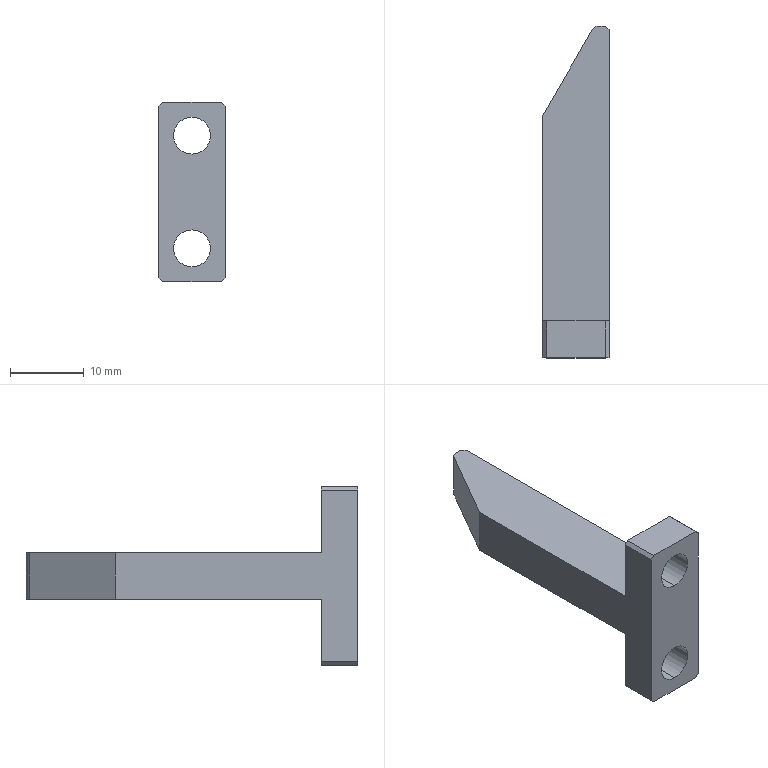Part | SolidWorks | features ICE 3, Chamfer 2, Extrusion 1, Fillet 1 | 1 solid | 21 faces | box 9 x 45 x 24.3 mm | volume 2894 mm3 | plane 16 | cylinder 5 | commonest cylinder face diameters 5 x4 2 x1
STEP:
#1=CARTESIAN_POINT('',(0.,-25.,8.3));
#2=VERTEX_POINT('',#1);
#3=CARTESIAN_POINT('',(0.,-25.,13.3));
#4=VERTEX_POINT('',#3);
#5=CARTESIAN_POINT('',(0.,-25.,10.8));
#6=DIRECTION('',(0.,1.,0.));
#7=DIRECTION('',(0.,0.,1.));
#8=AXIS2_PLACEMENT_3D('',#5,#6,#7);
#9=CIRCLE('',#8,2.5);
#10=EDGE_CURVE('',#2,#4,#9,.T.);
#11=ORIENTED_EDGE('',*,*,#10,.F.);
#12=CARTESIAN_POINT('',(0.,-20.,8.3));
#13=VERTEX_POINT('',#12);
#14=CARTESIAN_POINT('',(0.,-25.,8.3));
#15=DIRECTION('',(0.,1.,0.));
#16=VECTOR('',#15,1000.);
#17=LINE('',#14,#16);
#18=EDGE_CURVE('',#2,#13,#17,.T.);
#19=ORIENTED_EDGE('',*,*,#18,.T.);
#20=CARTESIAN_POINT('',(0.,-20.,13.3));
#21=VERTEX_POINT('',#20);
#22=CARTESIAN_POINT('',(0.,-20.,10.8));
#23=DIRECTION('',(0.,1.,0.));
#24=DIRECTION('',(0.,0.,1.));
#25=AXIS2_PLACEMENT_3D('',#22,#23,#24);
#26=CIRCLE('',#25,2.5);
#27=EDGE_CURVE('',#13,#21,#26,.T.);
#28=ORIENTED_EDGE('',*,*,#27,.T.);
#29=CARTESIAN_POINT('',(0.,-25.,13.3));
#30=DIRECTION('',(0.,1.,0.));
#31=VECTOR('',#30,1000.);
#32=LINE('',#29,#31);
#33=EDGE_CURVE('',#4,#21,#32,.T.);
#34=ORIENTED_EDGE('',*,*,#33,.F.);
#35=EDGE_LOOP('',(#11,#19,#28,#34));
#36=FACE_OUTER_BOUND('',#35,.T.);
#37=CARTESIAN_POINT('',(0.,-25.,10.8));
#38=DIRECTION('',(0.,1.,0.));
#39=DIRECTION('',(0.,0.,1.));
#40=AXIS2_PLACEMENT_3D('',#37,#38,#39);
#41=CYLINDRICAL_SURFACE('',#40,2.5);
#42=ADVANCED_FACE('',(#36),#41,.F.);
#43=CARTESIAN_POINT('',(0.,-25.,-7.));
#44=VERTEX_POINT('',#43);
#45=CARTESIAN_POINT('',(0.,-25.,-2.));
#46=VERTEX_POINT('',#45);
#47=CARTESIAN_POINT('',(0.,-25.,-4.5));
#48=DIRECTION('',(0.,1.,0.));
#49=DIRECTION('',(0.,0.,1.));
#50=AXIS2_PLACEMENT_3D('',#47,#48,#49);
#51=CIRCLE('',#50,2.5);
#52=EDGE_CURVE('',#44,#46,#51,.T.);
#53=ORIENTED_EDGE('',*,*,#52,.F.);
#54=CARTESIAN_POINT('',(0.,-20.,-7.));
#55=VERTEX_POINT('',#54);
#56=CARTESIAN_POINT('',(0.,-25.,-7.));
#57=DIRECTION('',(0.,1.,0.));
#58=VECTOR('',#57,1000.);
#59=LINE('',#56,#58);
#60=EDGE_CURVE('',#44,#55,#59,.T.);
#61=ORIENTED_EDGE('',*,*,#60,.T.);
#62=CARTESIAN_POINT('',(0.,-20.,-2.));
#63=VERTEX_POINT('',#62);
#64=CARTESIAN_POINT('',(0.,-20.,-4.5));
#65=DIRECTION('',(0.,1.,0.));
#66=DIRECTION('',(0.,0.,1.));
#67=AXIS2_PLACEMENT_3D('',#64,#65,#66);
#68=CIRCLE('',#67,2.5);
#69=EDGE_CURVE('',#55,#63,#68,.T.);
#70=ORIENTED_EDGE('',*,*,#69,.T.);
#71=CARTESIAN_POINT('',(0.,-25.,-2.));
#72=DIRECTION('',(0.,1.,0.));
#73=VECTOR('',#72,1000.);
#74=LINE('',#71,#73);
#75=EDGE_CURVE('',#46,#63,#74,.T.);
#76=ORIENTED_EDGE('',*,*,#75,.F.);
#77=EDGE_LOOP('',(#53,#61,#70,#76));
#78=FACE_OUTER_BOUND('',#77,.T.);
#79=CARTESIAN_POINT('',(0.,-25.,-4.5));
#80=DIRECTION('',(0.,1.,0.));
#81=DIRECTION('',(0.,0.,1.));
#82=AXIS2_PLACEMENT_3D('',#79,#80,#81);
#83=CYLINDRICAL_SURFACE('',#82,2.5);
#84=ADVANCED_FACE('',(#78),#83,.F.);
#85=CARTESIAN_POINT('',(4.5,-20.,0.));
#86=VERTEX_POINT('',#85);
#87=CARTESIAN_POINT('',(4.5,19.5,0.));
#88=VERTEX_POINT('',#87);
#89=CARTESIAN_POINT('',(4.5,20.,0.));
#90=DIRECTION('',(0.,1.,0.));
#91=VECTOR('',#90,1000.);
#92=LINE('',#89,#91);
#93=EDGE_CURVE('',#86,#88,#92,.T.);
#94=ORIENTED_EDGE('',*,*,#93,.T.);
#95=CARTESIAN_POINT('',(4.5,19.5,6.3));
#96=VERTEX_POINT('',#95);
#97=CARTESIAN_POINT('',(4.5,19.5,6.3));
#98=DIRECTION('',(0.,0.,1.));
#99=VECTOR('',#98,1000.);
#100=LINE('',#97,#99);
#101=EDGE_CURVE('',#88,#96,#100,.T.);
#102=ORIENTED_EDGE('',*,*,#101,.T.);
#103=CARTESIAN_POINT('',(4.5,-20.,6.3));
#104=VERTEX_POINT('',#103);
#105=CARTESIAN_POINT('',(4.5,20.,6.3));
#106=DIRECTION('',(0.,1.,0.));
#107=VECTOR('',#106,1000.);
#108=LINE('',#105,#107);
#109=EDGE_CURVE('',#104,#96,#108,.T.);
#110=ORIENTED_EDGE('',*,*,#109,.F.);
#111=CARTESIAN_POINT('',(4.5,-20.,14.8));
#112=VERTEX_POINT('',#111);
#113=CARTESIAN_POINT('',(4.5,-20.,15.3));
#114=DIRECTION('',(0.,0.,1.));
#115=VECTOR('',#114,1000.);
#116=LINE('',#113,#115);
#117=EDGE_CURVE('',#104,#112,#116,.T.);
#118=ORIENTED_EDGE('',*,*,#117,.T.);
#119=CARTESIAN_POINT('',(4.5,-25.,14.8));
#120=VERTEX_POINT('',#119);
#121=CARTESIAN_POINT('',(4.5,20.,14.8));
#122=DIRECTION('',(0.,-1.,0.));
#123=VECTOR('',#122,1000.);
#124=LINE('',#121,#123);
#125=EDGE_CURVE('',#112,#120,#124,.T.);
#126=ORIENTED_EDGE('',*,*,#125,.T.);
#127=CARTESIAN_POINT('',(4.5,-25.,-8.5));
#128=VERTEX_POINT('',#127);
#129=CARTESIAN_POINT('',(4.5,-25.,15.3));
#130=DIRECTION('',(0.,0.,1.));
#131=VECTOR('',#130,1000.);
#132=LINE('',#129,#131);
#133=EDGE_CURVE('',#128,#120,#132,.T.);
#134=ORIENTED_EDGE('',*,*,#133,.F.);
#135=CARTESIAN_POINT('',(4.5,-20.,-8.5));
#136=VERTEX_POINT('',#135);
#137=CARTESIAN_POINT('',(4.5,20.,-8.5));
#138=DIRECTION('',(0.,1.,0.));
#139=VECTOR('',#138,1000.);
#140=LINE('',#137,#139);
#141=EDGE_CURVE('',#128,#136,#140,.T.);
#142=ORIENTED_EDGE('',*,*,#141,.T.);
#143=CARTESIAN_POINT('',(4.5,-20.,15.3));
#144=DIRECTION('',(0.,0.,1.));
#145=VECTOR('',#144,1000.);
#146=LINE('',#143,#145);
#147=EDGE_CURVE('',#136,#86,#146,.T.);
#148=ORIENTED_EDGE('',*,*,#147,.T.);
#149=EDGE_LOOP('',(#94,#102,#110,#118,#126,#134,#142,#148));
#150=FACE_OUTER_BOUND('',#149,.T.);
#151=CARTESIAN_POINT('',(4.5,20.,6.3));
#152=DIRECTION('',(-1.,0.,0.));
#153=DIRECTION('',(0.,-1.,0.));
#154=AXIS2_PLACEMENT_3D('',#151,#152,#153);
#155=PLANE('',#154);
#156=ADVANCED_FACE('',(#150),#155,.F.);
#157=CARTESIAN_POINT('',(4.,20.,6.3));
#158=VERTEX_POINT('',#157);
#159=CARTESIAN_POINT('',(3.077,20.,6.3));
#160=VERTEX_POINT('',#159);
#161=CARTESIAN_POINT('',(-4.5,20.,6.3));
#162=DIRECTION('',(-1.,0.,0.));
#163=VECTOR('',#162,1000.);
#164=LINE('',#161,#163);
#165=EDGE_CURVE('',#158,#160,#164,.T.);
#166=ORIENTED_EDGE('',*,*,#165,.F.);
#167=CARTESIAN_POINT('',(4.,20.,0.));
#168=VERTEX_POINT('',#167);
#169=CARTESIAN_POINT('',(4.,20.,6.3));
#170=DIRECTION('',(0.,0.,-1.));
#171=VECTOR('',#170,1000.);
#172=LINE('',#169,#171);
#173=EDGE_CURVE('',#158,#168,#172,.T.);
#174=ORIENTED_EDGE('',*,*,#173,.T.);
#175=CARTESIAN_POINT('',(3.077,20.,0.));
#176=VERTEX_POINT('',#175);
#177=CARTESIAN_POINT('',(-4.5,20.,0.));
#178=DIRECTION('',(-1.,0.,0.));
#179=VECTOR('',#178,1000.);
#180=LINE('',#177,#179);
#181=EDGE_CURVE('',#168,#176,#180,.T.);
#182=ORIENTED_EDGE('',*,*,#181,.T.);
#183=CARTESIAN_POINT('',(3.077,20.,6.3));
#184=DIRECTION('',(0.,0.,1.));
#185=VECTOR('',#184,1000.);
#186=LINE('',#183,#185);
#187=EDGE_CURVE('',#176,#160,#186,.T.);
#188=ORIENTED_EDGE('',*,*,#187,.T.);
#189=EDGE_LOOP('',(#166,#174,#182,#188));
#190=FACE_OUTER_BOUND('',#189,.T.);
#191=CARTESIAN_POINT('',(-4.5,20.,6.3));
#192=DIRECTION('',(0.,-1.,0.));
#193=DIRECTION('',(0.,0.,-1.));
#194=AXIS2_PLACEMENT_3D('',#191,#192,#193);
#195=PLANE('',#194);
#196=ADVANCED_FACE('',(#190),#195,.F.);
#197=CARTESIAN_POINT('',(-4.5,-20.,0.));
#198=VERTEX_POINT('',#197);
#199=CARTESIAN_POINT('',(-4.5,-20.,-8.5));
#200=VERTEX_POINT('',#199);
#201=CARTESIAN_POINT('',(-4.5,-20.,15.3));
#202=DIRECTION('',(0.,0.,-1.));
#203=VECTOR('',#202,1000.);
#204=LINE('',#201,#203);
#205=EDGE_CURVE('',#198,#200,#204,.T.);
#206=ORIENTED_EDGE('',*,*,#205,.T.);
#207=CARTESIAN_POINT('',(-4.5,-25.,-8.5));
#208=VERTEX_POINT('',#207);
#209=CARTESIAN_POINT('',(-4.5,20.,-8.5));
#210=DIRECTION('',(0.,-1.,0.));
#211=VECTOR('',#210,1000.);
#212=LINE('',#209,#211);
#213=EDGE_CURVE('',#200,#208,#212,.T.);
#214=ORIENTED_EDGE('',*,*,#213,.T.);
#215=CARTESIAN_POINT('',(-4.5,-25.,14.8));
#216=VERTEX_POINT('',#215);
#217=CARTESIAN_POINT('',(-4.5,-25.,15.3));
#218=DIRECTION('',(0.,0.,-1.));
#219=VECTOR('',#218,1000.);
#220=LINE('',#217,#219);
#221=EDGE_CURVE('',#216,#208,#220,.T.);
#222=ORIENTED_EDGE('',*,*,#221,.F.);
#223=CARTESIAN_POINT('',(-4.5,-20.,14.8));
#224=VERTEX_POINT('',#223);
#225=CARTESIAN_POINT('',(-4.5,20.,14.8));
#226=DIRECTION('',(0.,1.,0.));
#227=VECTOR('',#226,1000.);
#228=LINE('',#225,#227);
#229=EDGE_CURVE('',#216,#224,#228,.T.);
#230=ORIENTED_EDGE('',*,*,#229,.T.);
#231=CARTESIAN_POINT('',(-4.5,-20.,6.3));
#232=VERTEX_POINT('',#231);
#233=CARTESIAN_POINT('',(-4.5,-20.,15.3));
#234=DIRECTION('',(0.,0.,-1.));
#235=VECTOR('',#234,1000.);
#236=LINE('',#233,#235);
#237=EDGE_CURVE('',#224,#232,#236,.T.);
#238=ORIENTED_EDGE('',*,*,#237,.T.);
#239=CARTESIAN_POINT('',(-4.5,7.876,6.3));
#240=VERTEX_POINT('',#239);
#241=CARTESIAN_POINT('',(-4.5,20.,6.3));
#242=DIRECTION('',(0.,-1.,0.));
#243=VECTOR('',#242,1000.);
#244=LINE('',#241,#243);
#245=EDGE_CURVE('',#240,#232,#244,.T.);
#246=ORIENTED_EDGE('',*,*,#245,.F.);
#247=CARTESIAN_POINT('',(-4.5,7.876,0.));
#248=VERTEX_POINT('',#247);
#249=CARTESIAN_POINT('',(-4.5,7.876,15.3));
#250=DIRECTION('',(0.,0.,-1.));
#251=VECTOR('',#250,1000.);
#252=LINE('',#249,#251);
#253=EDGE_CURVE('',#240,#248,#252,.T.);
#254=ORIENTED_EDGE('',*,*,#253,.T.);
#255=CARTESIAN_POINT('',(-4.5,20.,0.));
#256=DIRECTION('',(0.,-1.,0.));
#257=VECTOR('',#256,1000.);
#258=LINE('',#255,#257);
#259=EDGE_CURVE('',#248,#198,#258,.T.);
#260=ORIENTED_EDGE('',*,*,#259,.T.);
#261=EDGE_LOOP('',(#206,#214,#222,#230,#238,#246,#254,#260));
#262=FACE_OUTER_BOUND('',#261,.T.);
#263=CARTESIAN_POINT('',(-4.5,20.,6.3));
#264=DIRECTION('',(1.,0.,0.));
#265=DIRECTION('',(0.,1.,0.));
#266=AXIS2_PLACEMENT_3D('',#263,#264,#265);
#267=PLANE('',#266);
#268=ADVANCED_FACE('',(#262),#267,.F.);
#269=ORIENTED_EDGE('',*,*,#109,.T.);
#270=CARTESIAN_POINT('',(12.,12.,6.3));
#271=DIRECTION('',(-0.7071,0.7071,0.));
#272=VECTOR('',#271,1000.);
#273=LINE('',#270,#272);
#274=EDGE_CURVE('',#96,#158,#273,.T.);
#275=ORIENTED_EDGE('',*,*,#274,.T.);
#276=ORIENTED_EDGE('',*,*,#165,.T.);
#277=CARTESIAN_POINT('',(2.211,19.5,6.3));
#278=VERTEX_POINT('',#277);
#279=CARTESIAN_POINT('',(3.077,19.,6.3));
#280=DIRECTION('',(0.,0.,1.));
#281=DIRECTION('',(1.,0.,0.));
#282=AXIS2_PLACEMENT_3D('',#279,#280,#281);
#283=CIRCLE('',#282,1.);
#284=EDGE_CURVE('',#160,#278,#283,.T.);
#285=ORIENTED_EDGE('',*,*,#284,.T.);
#286=CARTESIAN_POINT('',(-6.785,3.917,6.3));
#287=DIRECTION('',(0.5,0.866,0.));
#288=VECTOR('',#287,1000.);
#289=LINE('',#286,#288);
#290=EDGE_CURVE('',#240,#278,#289,.T.);
#291=ORIENTED_EDGE('',*,*,#290,.F.);
#292=ORIENTED_EDGE('',*,*,#245,.T.);
#293=CARTESIAN_POINT('',(-4.5,-20.,6.3));
#294=DIRECTION('',(1.,0.,0.));
#295=VECTOR('',#294,1000.);
#296=LINE('',#293,#295);
#297=EDGE_CURVE('',#232,#104,#296,.T.);
#298=ORIENTED_EDGE('',*,*,#297,.T.);
#299=EDGE_LOOP('',(#269,#275,#276,#285,#291,#292,#298));
#300=FACE_OUTER_BOUND('',#299,.T.);
#301=CARTESIAN_POINT('',(0.,0.,6.3));
#302=DIRECTION('',(0.,0.,1.));
#303=DIRECTION('',(1.,0.,0.));
#304=AXIS2_PLACEMENT_3D('',#301,#302,#303);
#305=PLANE('',#304);
#306=ADVANCED_FACE('',(#300),#305,.T.);
#307=ORIENTED_EDGE('',*,*,#181,.F.);
#308=CARTESIAN_POINT('',(4.,20.,0.));
#309=DIRECTION('',(0.7071,-0.7071,0.));
#310=VECTOR('',#309,1000.);
#311=LINE('',#308,#310);
#312=EDGE_CURVE('',#168,#88,#311,.T.);
#313=ORIENTED_EDGE('',*,*,#312,.T.);
#314=ORIENTED_EDGE('',*,*,#93,.F.);
#315=CARTESIAN_POINT('',(-4.5,-20.,0.));
#316=DIRECTION('',(1.,0.,0.));
#317=VECTOR('',#316,1000.);
#318=LINE('',#315,#317);
#319=EDGE_CURVE('',#198,#86,#318,.T.);
#320=ORIENTED_EDGE('',*,*,#319,.F.);
#321=ORIENTED_EDGE('',*,*,#259,.F.);
#322=CARTESIAN_POINT('',(2.211,19.5,0.));
#323=VERTEX_POINT('',#322);
#324=CARTESIAN_POINT('',(-4.5,7.876,0.));
#325=DIRECTION('',(-0.5,-0.866,0.));
#326=VECTOR('',#325,1000.);
#327=LINE('',#324,#326);
#328=EDGE_CURVE('',#323,#248,#327,.T.);
#329=ORIENTED_EDGE('',*,*,#328,.F.);
#330=CARTESIAN_POINT('',(3.077,19.,0.));
#331=DIRECTION('',(0.,0.,-1.));
#332=DIRECTION('',(1.,0.,0.));
#333=AXIS2_PLACEMENT_3D('',#330,#331,#332);
#334=CIRCLE('',#333,1.);
#335=EDGE_CURVE('',#323,#176,#334,.T.);
#336=ORIENTED_EDGE('',*,*,#335,.T.);
#337=EDGE_LOOP('',(#307,#313,#314,#320,#321,#329,#336));
#338=FACE_OUTER_BOUND('',#337,.T.);
#339=CARTESIAN_POINT('',(0.,0.,0.));
#340=DIRECTION('',(0.,0.,1.));
#341=DIRECTION('',(1.,0.,0.));
#342=AXIS2_PLACEMENT_3D('',#339,#340,#341);
#343=PLANE('',#342);
#344=ADVANCED_FACE('',(#338),#343,.F.);
#345=CARTESIAN_POINT('',(0.,-20.,-4.5));
#346=DIRECTION('',(0.,1.,0.));
#347=DIRECTION('',(0.,0.,1.));
#348=AXIS2_PLACEMENT_3D('',#345,#346,#347);
#349=CIRCLE('',#348,2.5);
#350=EDGE_CURVE('',#63,#55,#349,.T.);
#351=ORIENTED_EDGE('',*,*,#350,.F.);
#352=ORIENTED_EDGE('',*,*,#69,.F.);
#353=EDGE_LOOP('',(#351,#352));
#354=FACE_BOUND('',#353,.T.);
#355=ORIENTED_EDGE('',*,*,#147,.F.);
#356=CARTESIAN_POINT('',(4.,-20.,-9.));
#357=VERTEX_POINT('',#356);
#358=CARTESIAN_POINT('',(4.5,-20.,-8.5));
#359=DIRECTION('',(-0.7071,0.,-0.7071));
#360=VECTOR('',#359,1000.);
#361=LINE('',#358,#360);
#362=EDGE_CURVE('',#136,#357,#361,.T.);
#363=ORIENTED_EDGE('',*,*,#362,.T.);
#364=CARTESIAN_POINT('',(-4.,-20.,-9.));
#365=VERTEX_POINT('',#364);
#366=CARTESIAN_POINT('',(-4.5,-20.,-9.));
#367=DIRECTION('',(1.,0.,0.));
#368=VECTOR('',#367,1000.);
#369=LINE('',#366,#368);
#370=EDGE_CURVE('',#365,#357,#369,.T.);
#371=ORIENTED_EDGE('',*,*,#370,.F.);
#372=CARTESIAN_POINT('',(-4.,-20.,-9.));
#373=DIRECTION('',(-0.7071,0.,0.7071));
#374=VECTOR('',#373,1000.);
#375=LINE('',#372,#374);
#376=EDGE_CURVE('',#365,#200,#375,.T.);
#377=ORIENTED_EDGE('',*,*,#376,.T.);
#378=ORIENTED_EDGE('',*,*,#205,.F.);
#379=ORIENTED_EDGE('',*,*,#319,.T.);
#380=EDGE_LOOP('',(#355,#363,#371,#377,#378,#379));
#381=FACE_OUTER_BOUND('',#380,.T.);
#382=CARTESIAN_POINT('',(0.,-20.,0.));
#383=DIRECTION('',(0.,-1.,0.));
#384=DIRECTION('',(0.,0.,-1.));
#385=AXIS2_PLACEMENT_3D('',#382,#383,#384);
#386=PLANE('',#385);
#387=ADVANCED_FACE('',(#354,#381),#386,.F.);
#388=ORIENTED_EDGE('',*,*,#370,.T.);
#389=CARTESIAN_POINT('',(4.,-25.,-9.));
#390=VERTEX_POINT('',#389);
#391=CARTESIAN_POINT('',(4.,-25.,-9.));
#392=DIRECTION('',(0.,-1.,0.));
#393=VECTOR('',#392,1000.);
#394=LINE('',#391,#393);
#395=EDGE_CURVE('',#357,#390,#394,.T.);
#396=ORIENTED_EDGE('',*,*,#395,.T.);
#397=CARTESIAN_POINT('',(-4.,-25.,-9.));
#398=VERTEX_POINT('',#397);
#399=CARTESIAN_POINT('',(-4.5,-25.,-9.));
#400=DIRECTION('',(1.,0.,0.));
#401=VECTOR('',#400,1000.);
#402=LINE('',#399,#401);
#403=EDGE_CURVE('',#398,#390,#402,.T.);
#404=ORIENTED_EDGE('',*,*,#403,.F.);
#405=CARTESIAN_POINT('',(-4.,-25.,-9.));
#406=DIRECTION('',(0.,1.,0.));
#407=VECTOR('',#406,1000.);
#408=LINE('',#405,#407);
#409=EDGE_CURVE('',#398,#365,#408,.T.);
#410=ORIENTED_EDGE('',*,*,#409,.T.);
#411=EDGE_LOOP('',(#388,#396,#404,#410));
#412=FACE_OUTER_BOUND('',#411,.T.);
#413=CARTESIAN_POINT('',(-4.5,-25.,-9.));
#414=DIRECTION('',(0.,0.,1.));
#415=DIRECTION('',(1.,0.,0.));
#416=AXIS2_PLACEMENT_3D('',#413,#414,#415);
#417=PLANE('',#416);
#418=ADVANCED_FACE('',(#412),#417,.F.);
#419=CARTESIAN_POINT('',(4.,-25.,15.3));
#420=VERTEX_POINT('',#419);
#421=CARTESIAN_POINT('',(-4.,-25.,15.3));
#422=VERTEX_POINT('',#421);
#423=CARTESIAN_POINT('',(-4.5,-25.,15.3));
#424=DIRECTION('',(-1.,0.,0.));
#425=VECTOR('',#424,1000.);
#426=LINE('',#423,#425);
#427=EDGE_CURVE('',#420,#422,#426,.T.);
#428=ORIENTED_EDGE('',*,*,#427,.F.);
#429=CARTESIAN_POINT('',(4.,-20.,15.3));
#430=VERTEX_POINT('',#429);
#431=CARTESIAN_POINT('',(4.,-25.,15.3));
#432=DIRECTION('',(0.,1.,0.));
#433=VECTOR('',#432,1000.);
#434=LINE('',#431,#433);
#435=EDGE_CURVE('',#420,#430,#434,.T.);
#436=ORIENTED_EDGE('',*,*,#435,.T.);
#437=CARTESIAN_POINT('',(-4.,-20.,15.3));
#438=VERTEX_POINT('',#437);
#439=CARTESIAN_POINT('',(-4.5,-20.,15.3));
#440=DIRECTION('',(-1.,0.,0.));
#441=VECTOR('',#440,1000.);
#442=LINE('',#439,#441);
#443=EDGE_CURVE('',#430,#438,#442,.T.);
#444=ORIENTED_EDGE('',*,*,#443,.T.);
#445=CARTESIAN_POINT('',(-4.,-25.,15.3));
#446=DIRECTION('',(0.,-1.,0.));
#447=VECTOR('',#446,1000.);
#448=LINE('',#445,#447);
#449=EDGE_CURVE('',#438,#422,#448,.T.);
#450=ORIENTED_EDGE('',*,*,#449,.T.);
#451=EDGE_LOOP('',(#428,#436,#444,#450));
#452=FACE_OUTER_BOUND('',#451,.T.);
#453=CARTESIAN_POINT('',(-4.5,-25.,15.3));
#454=DIRECTION('',(0.,0.,-1.));
#455=DIRECTION('',(-1.,0.,0.));
#456=AXIS2_PLACEMENT_3D('',#453,#454,#455);
#457=PLANE('',#456);
#458=ADVANCED_FACE('',(#452),#457,.F.);
#459=CARTESIAN_POINT('',(0.,-25.,10.8));
#460=DIRECTION('',(0.,1.,0.));
#461=DIRECTION('',(0.,0.,1.));
#462=AXIS2_PLACEMENT_3D('',#459,#460,#461);
#463=CIRCLE('',#462,2.5);
#464=EDGE_CURVE('',#4,#2,#463,.T.);
#465=ORIENTED_EDGE('',*,*,#464,.T.);
#466=ORIENTED_EDGE('',*,*,#10,.T.);
#467=EDGE_LOOP('',(#465,#466));
#468=FACE_BOUND('',#467,.T.);
#469=CARTESIAN_POINT('',(0.,-25.,-4.5));
#470=DIRECTION('',(0.,1.,0.));
#471=DIRECTION('',(0.,0.,1.));
#472=AXIS2_PLACEMENT_3D('',#469,#470,#471);
#473=CIRCLE('',#472,2.5);
#474=EDGE_CURVE('',#46,#44,#473,.T.);
#475=ORIENTED_EDGE('',*,*,#474,.T.);
#476=ORIENTED_EDGE('',*,*,#52,.T.);
#477=EDGE_LOOP('',(#475,#476));
#478=FACE_BOUND('',#477,.T.);
#479=ORIENTED_EDGE('',*,*,#403,.T.);
#480=CARTESIAN_POINT('',(6.5,-25.,-6.5));
#481=DIRECTION('',(0.7071,0.,0.7071));
#482=VECTOR('',#481,1000.);
#483=LINE('',#480,#482);
#484=EDGE_CURVE('',#390,#128,#483,.T.);
#485=ORIENTED_EDGE('',*,*,#484,.T.);
#486=ORIENTED_EDGE('',*,*,#133,.T.);
#487=CARTESIAN_POINT('',(9.65,-25.,9.65));
#488=DIRECTION('',(-0.7071,0.,0.7071));
#489=VECTOR('',#488,1000.);
#490=LINE('',#487,#489);
#491=EDGE_CURVE('',#120,#420,#490,.T.);
#492=ORIENTED_EDGE('',*,*,#491,.T.);
#493=ORIENTED_EDGE('',*,*,#427,.T.);
#494=CARTESIAN_POINT('',(-9.65,-25.,9.65));
#495=DIRECTION('',(-0.7071,0.,-0.7071));
#496=VECTOR('',#495,1000.);
#497=LINE('',#494,#496);
#498=EDGE_CURVE('',#422,#216,#497,.T.);
#499=ORIENTED_EDGE('',*,*,#498,.T.);
#500=ORIENTED_EDGE('',*,*,#221,.T.);
#501=CARTESIAN_POINT('',(-6.5,-25.,-6.5));
#502=DIRECTION('',(0.7071,0.,-0.7071));
#503=VECTOR('',#502,1000.);
#504=LINE('',#501,#503);
#505=EDGE_CURVE('',#208,#398,#504,.T.);
#506=ORIENTED_EDGE('',*,*,#505,.T.);
#507=EDGE_LOOP('',(#479,#485,#486,#492,#493,#499,#500,#506));
#508=FACE_OUTER_BOUND('',#507,.T.);
#509=CARTESIAN_POINT('',(0.,-25.,0.));
#510=DIRECTION('',(0.,-1.,0.));
#511=DIRECTION('',(0.,0.,-1.));
#512=AXIS2_PLACEMENT_3D('',#509,#510,#511);
#513=PLANE('',#512);
#514=ADVANCED_FACE('',(#468,#478,#508),#513,.T.);
#515=CARTESIAN_POINT('',(0.,-20.,10.8));
#516=DIRECTION('',(0.,1.,0.));
#517=DIRECTION('',(0.,0.,1.));
#518=AXIS2_PLACEMENT_3D('',#515,#516,#517);
#519=CIRCLE('',#518,2.5);
#520=EDGE_CURVE('',#21,#13,#519,.T.);
#521=ORIENTED_EDGE('',*,*,#520,.F.);
#522=ORIENTED_EDGE('',*,*,#27,.F.);
#523=EDGE_LOOP('',(#521,#522));
#524=FACE_BOUND('',#523,.T.);
#525=ORIENTED_EDGE('',*,*,#443,.F.);
#526=CARTESIAN_POINT('',(4.,-20.,15.3));
#527=DIRECTION('',(0.7071,0.,-0.7071));
#528=VECTOR('',#527,1000.);
#529=LINE('',#526,#528);
#530=EDGE_CURVE('',#430,#112,#529,.T.);
#531=ORIENTED_EDGE('',*,*,#530,.T.);
#532=ORIENTED_EDGE('',*,*,#117,.F.);
#533=ORIENTED_EDGE('',*,*,#297,.F.);
#534=ORIENTED_EDGE('',*,*,#237,.F.);
#535=CARTESIAN_POINT('',(-4.5,-20.,14.8));
#536=DIRECTION('',(0.7071,0.,0.7071));
#537=VECTOR('',#536,1000.);
#538=LINE('',#535,#537);
#539=EDGE_CURVE('',#224,#438,#538,.T.);
#540=ORIENTED_EDGE('',*,*,#539,.T.);
#541=EDGE_LOOP('',(#525,#531,#532,#533,#534,#540));
#542=FACE_OUTER_BOUND('',#541,.T.);
#543=CARTESIAN_POINT('',(0.,-20.,0.));
#544=DIRECTION('',(0.,-1.,0.));
#545=DIRECTION('',(0.,0.,-1.));
#546=AXIS2_PLACEMENT_3D('',#543,#544,#545);
#547=PLANE('',#546);
#548=ADVANCED_FACE('',(#524,#542),#547,.F.);
#549=ORIENTED_EDGE('',*,*,#290,.T.);
#550=CARTESIAN_POINT('',(2.211,19.5,15.3));
#551=DIRECTION('',(0.,0.,-1.));
#552=VECTOR('',#551,1000.);
#553=LINE('',#550,#552);
#554=EDGE_CURVE('',#278,#323,#553,.T.);
#555=ORIENTED_EDGE('',*,*,#554,.T.);
#556=ORIENTED_EDGE('',*,*,#328,.T.);
#557=ORIENTED_EDGE('',*,*,#253,.F.);
#558=EDGE_LOOP('',(#549,#555,#556,#557));
#559=FACE_OUTER_BOUND('',#558,.T.);
#560=CARTESIAN_POINT('',(-4.5,7.876,15.3));
#561=DIRECTION('',(0.866,-0.5,0.));
#562=DIRECTION('',(0.5,0.866,0.));
#563=AXIS2_PLACEMENT_3D('',#560,#561,#562);
#564=PLANE('',#563);
#565=ADVANCED_FACE('',(#559),#564,.F.);
#566=ORIENTED_EDGE('',*,*,#60,.F.);
#567=ORIENTED_EDGE('',*,*,#474,.F.);
#568=ORIENTED_EDGE('',*,*,#75,.T.);
#569=ORIENTED_EDGE('',*,*,#350,.T.);
#570=EDGE_LOOP('',(#566,#567,#568,#569));
#571=FACE_OUTER_BOUND('',#570,.T.);
#572=CARTESIAN_POINT('',(0.,-25.,-4.5));
#573=DIRECTION('',(0.,1.,0.));
#574=DIRECTION('',(0.,0.,1.));
#575=AXIS2_PLACEMENT_3D('',#572,#573,#574);
#576=CYLINDRICAL_SURFACE('',#575,2.5);
#577=ADVANCED_FACE('',(#571),#576,.F.);
#578=ORIENTED_EDGE('',*,*,#18,.F.);
#579=ORIENTED_EDGE('',*,*,#464,.F.);
#580=ORIENTED_EDGE('',*,*,#33,.T.);
#581=ORIENTED_EDGE('',*,*,#520,.T.);
#582=EDGE_LOOP('',(#578,#579,#580,#581));
#583=FACE_OUTER_BOUND('',#582,.T.);
#584=CARTESIAN_POINT('',(0.,-25.,10.8));
#585=DIRECTION('',(0.,1.,0.));
#586=DIRECTION('',(0.,0.,1.));
#587=AXIS2_PLACEMENT_3D('',#584,#585,#586);
#588=CYLINDRICAL_SURFACE('',#587,2.5);
#589=ADVANCED_FACE('',(#583),#588,.F.);
#590=ORIENTED_EDGE('',*,*,#284,.F.);
#591=ORIENTED_EDGE('',*,*,#187,.F.);
#592=ORIENTED_EDGE('',*,*,#335,.F.);
#593=ORIENTED_EDGE('',*,*,#554,.F.);
#594=EDGE_LOOP('',(#590,#591,#592,#593));
#595=FACE_OUTER_BOUND('',#594,.T.);
#596=CARTESIAN_POINT('',(3.077,19.,15.3));
#597=DIRECTION('',(0.,0.,-1.));
#598=DIRECTION('',(-1.,0.,0.));
#599=AXIS2_PLACEMENT_3D('',#596,#597,#598);
#600=CYLINDRICAL_SURFACE('',#599,1.);
#601=ADVANCED_FACE('',(#595),#600,.T.);
#602=ORIENTED_EDGE('',*,*,#274,.F.);
#603=ORIENTED_EDGE('',*,*,#101,.F.);
#604=ORIENTED_EDGE('',*,*,#312,.F.);
#605=ORIENTED_EDGE('',*,*,#173,.F.);
#606=EDGE_LOOP('',(#602,#603,#604,#605));
#607=FACE_OUTER_BOUND('',#606,.T.);
#608=CARTESIAN_POINT('',(4.,20.,6.3));
#609=DIRECTION('',(-0.7071,-0.7071,0.));
#610=DIRECTION('',(0.,0.,-1.));
#611=AXIS2_PLACEMENT_3D('',#608,#609,#610);
#612=PLANE('',#611);
#613=ADVANCED_FACE('',(#607),#612,.F.);
#614=ORIENTED_EDGE('',*,*,#484,.F.);
#615=ORIENTED_EDGE('',*,*,#395,.F.);
#616=ORIENTED_EDGE('',*,*,#362,.F.);
#617=ORIENTED_EDGE('',*,*,#141,.F.);
#618=EDGE_LOOP('',(#614,#615,#616,#617));
#619=FACE_OUTER_BOUND('',#618,.T.);
#620=CARTESIAN_POINT('',(4.5,20.,-8.5));
#621=DIRECTION('',(-0.7071,0.,0.7071));
#622=DIRECTION('',(0.,1.,0.));
#623=AXIS2_PLACEMENT_3D('',#620,#621,#622);
#624=PLANE('',#623);
#625=ADVANCED_FACE('',(#619),#624,.F.);
#626=ORIENTED_EDGE('',*,*,#505,.F.);
#627=ORIENTED_EDGE('',*,*,#213,.F.);
#628=ORIENTED_EDGE('',*,*,#376,.F.);
#629=ORIENTED_EDGE('',*,*,#409,.F.);
#630=EDGE_LOOP('',(#626,#627,#628,#629));
#631=FACE_OUTER_BOUND('',#630,.T.);
#632=CARTESIAN_POINT('',(-4.,-25.,-9.));
#633=DIRECTION('',(0.7071,0.,0.7071));
#634=DIRECTION('',(0.,1.,0.));
#635=AXIS2_PLACEMENT_3D('',#632,#633,#634);
#636=PLANE('',#635);
#637=ADVANCED_FACE('',(#631),#636,.F.);
#638=ORIENTED_EDGE('',*,*,#491,.F.);
#639=ORIENTED_EDGE('',*,*,#125,.F.);
#640=ORIENTED_EDGE('',*,*,#530,.F.);
#641=ORIENTED_EDGE('',*,*,#435,.F.);
#642=EDGE_LOOP('',(#638,#639,#640,#641));
#643=FACE_OUTER_BOUND('',#642,.T.);
#644=CARTESIAN_POINT('',(4.,-25.,15.3));
#645=DIRECTION('',(-0.7071,0.,-0.7071));
#646=DIRECTION('',(0.,1.,0.));
#647=AXIS2_PLACEMENT_3D('',#644,#645,#646);
#648=PLANE('',#647);
#649=ADVANCED_FACE('',(#643),#648,.F.);
#650=ORIENTED_EDGE('',*,*,#498,.F.);
#651=ORIENTED_EDGE('',*,*,#449,.F.);
#652=ORIENTED_EDGE('',*,*,#539,.F.);
#653=ORIENTED_EDGE('',*,*,#229,.F.);
#654=EDGE_LOOP('',(#650,#651,#652,#653));
#655=FACE_OUTER_BOUND('',#654,.T.);
#656=CARTESIAN_POINT('',(-4.5,20.,14.8));
#657=DIRECTION('',(0.7071,0.,-0.7071));
#658=DIRECTION('',(0.,1.,0.));
#659=AXIS2_PLACEMENT_3D('',#656,#657,#658);
#660=PLANE('',#659);
#661=ADVANCED_FACE('',(#655),#660,.F.);
#662=CLOSED_SHELL('',(#42,#84,#156,#196,#268,#306,#344,#387,#418,#458,#514,#548,#565,#577,#589,#601,#613,#625,#637,#649,#661));
#663=MANIFOLD_SOLID_BREP('',#662);
#664=CARTESIAN_POINT('',(0.,0.,0.));
#665=DIRECTION('',(0.,0.,1.));
#666=DIRECTION('',(1.,0.,0.));
#667=AXIS2_PLACEMENT_3D('',#664,#665,#666);
#668=(LENGTH_UNIT()NAMED_UNIT(*)SI_UNIT(.MILLI.,.METRE.));
#669=UNCERTAINTY_MEASURE_WITH_UNIT(LENGTH_MEASURE(0.00001),#668,'','');
#670=(NAMED_UNIT(*)PLANE_ANGLE_UNIT()SI_UNIT($,.RADIAN.));
#671=(NAMED_UNIT(*)SI_UNIT($,.STERADIAN.)SOLID_ANGLE_UNIT());
#672=(GEOMETRIC_REPRESENTATION_CONTEXT(3)GLOBAL_UNCERTAINTY_ASSIGNED_CONTEXT((#669))GLOBAL_UNIT_ASSIGNED_CONTEXT((#668,#670,#671))REPRESENTATION_CONTEXT('',''));
#673=ADVANCED_BREP_SHAPE_REPRESENTATION('',(#663,#667),#672);